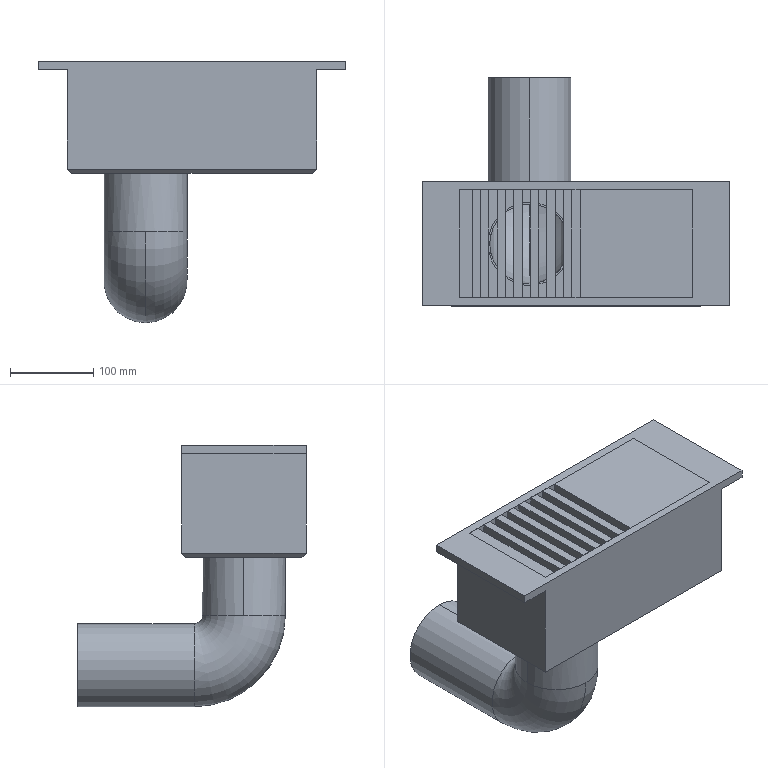Part | SolidWorks | features ICE 6, Shell 2, Chamfer 1, Extrusion 1, LPattern 1, Sweep 1 | 10 solids | 83 faces | box 370 x 275 x 315 mm | volume 2000718 mm3 | plane 69 | cylinder 10 | torus 4 | commonest cylinder face diameters 100 x6 96 x4